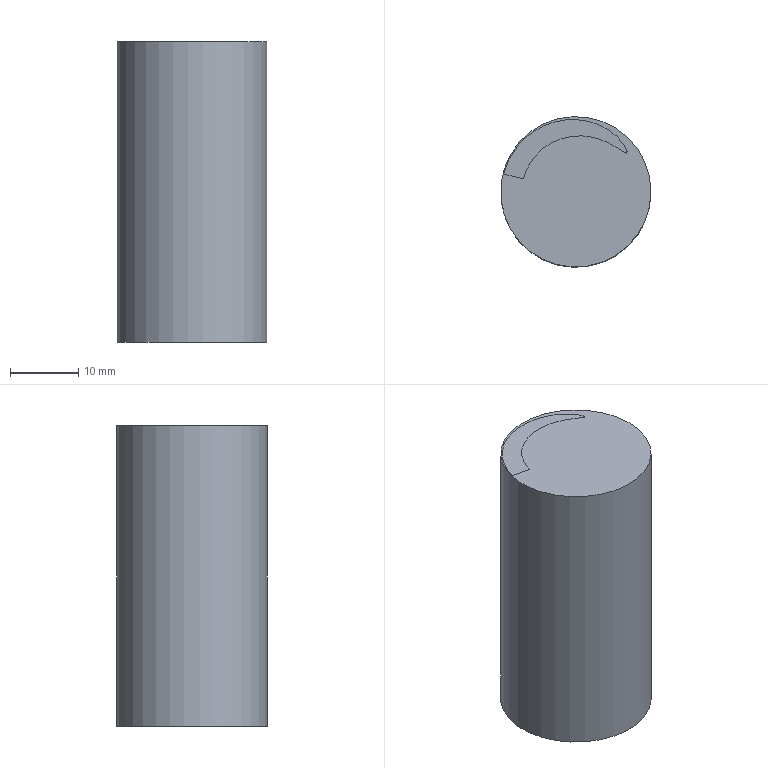Part | NX | features BREP 2 | 2 solids | 8 faces | box 22 x 22 x 44 mm | volume 20923 mm3 | plane 6 | cylinder 1 | spline 1 | commonest cylinder face diameters 22 x1